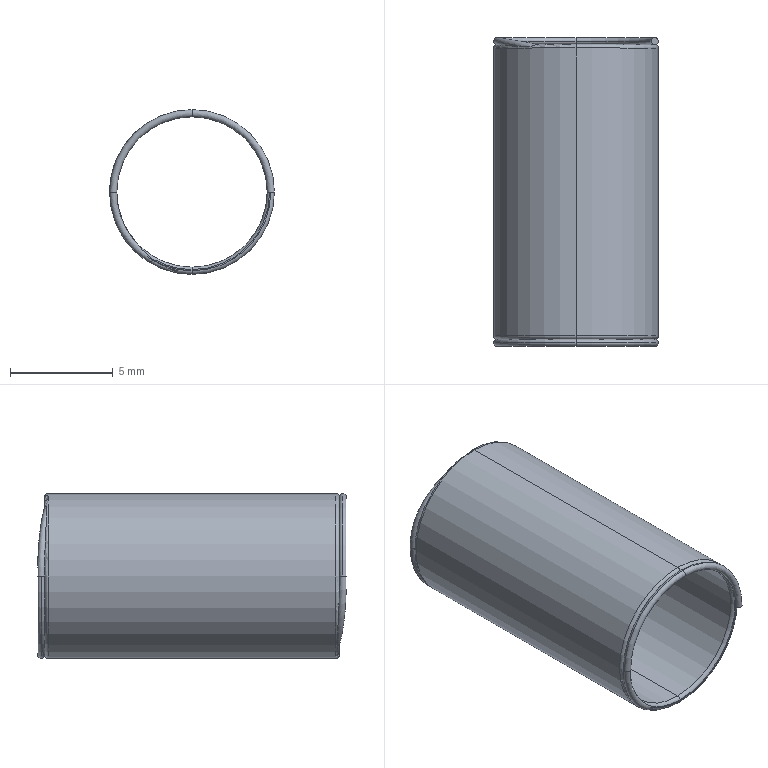Part | STEP file | 11-UF8-15-A11_UV8-15 | 1 solid | 30 faces | box 8 x 15 x 8 mm | volume 122.558 mm3 | torus 22 | cylinder 4 | plane 4 | commonest cylinder face diameters 7.3 x2 8 x2
STEP:
#1=CARTESIAN_POINT('',(0.,-7.325,4.));
#2=VERTEX_POINT('',#1);
#3=CARTESIAN_POINT('',(0.,-7.325,3.65));
#4=VERTEX_POINT('',#3);
#5=CARTESIAN_POINT('',(0.,-7.325,3.825));
#6=DIRECTION('',(1.,0.,0.));
#7=DIRECTION('',(0.,0.,-1.));
#8=AXIS2_PLACEMENT_3D('',#5,#6,#7);
#9=CIRCLE('',#8,0.175);
#10=EDGE_CURVE('',#2,#4,#9,.T.);
#11=ORIENTED_EDGE('',*,*,#10,.F.);
#12=CARTESIAN_POINT('',(-4.,-7.325,0.));
#13=VERTEX_POINT('',#12);
#14=CARTESIAN_POINT('',(0.,-7.325,0.));
#15=DIRECTION('',(0.,-1.,0.));
#16=DIRECTION('',(0.,0.,-1.));
#17=AXIS2_PLACEMENT_3D('',#14,#15,#16);
#18=CIRCLE('',#17,4.);
#19=EDGE_CURVE('',#2,#13,#18,.T.);
#20=ORIENTED_EDGE('',*,*,#19,.T.);
#21=CARTESIAN_POINT('',(-3.65,-7.325,0.));
#22=VERTEX_POINT('',#21);
#23=CARTESIAN_POINT('',(-3.825,-7.325,0.));
#24=DIRECTION('',(0.,0.,1.));
#25=DIRECTION('',(1.,0.,0.));
#26=AXIS2_PLACEMENT_3D('',#23,#24,#25);
#27=CIRCLE('',#26,0.175);
#28=EDGE_CURVE('',#13,#22,#27,.T.);
#29=ORIENTED_EDGE('',*,*,#28,.T.);
#30=CARTESIAN_POINT('',(0.,-7.325,0.));
#31=DIRECTION('',(0.,-1.,0.));
#32=DIRECTION('',(0.,0.,-1.));
#33=AXIS2_PLACEMENT_3D('',#30,#31,#32);
#34=CIRCLE('',#33,3.65);
#35=EDGE_CURVE('',#4,#22,#34,.T.);
#36=ORIENTED_EDGE('',*,*,#35,.F.);
#37=EDGE_LOOP('',(#11,#20,#29,#36));
#38=FACE_OUTER_BOUND('',#37,.T.);
#39=CARTESIAN_POINT('',(0.,-7.325,0.));
#40=DIRECTION('',(0.,-1.,0.));
#41=DIRECTION('',(0.,0.,-1.));
#42=AXIS2_PLACEMENT_3D('',#39,#40,#41);
#43=TOROIDAL_SURFACE('',#42,3.825,0.175);
#44=ADVANCED_FACE('',(#38),#43,.T.);
#45=CARTESIAN_POINT('',(0.,-7.15,3.825));
#46=VERTEX_POINT('',#45);
#47=CARTESIAN_POINT('',(0.,-7.325,3.825));
#48=DIRECTION('',(1.,0.,0.));
#49=DIRECTION('',(0.,0.,-1.));
#50=AXIS2_PLACEMENT_3D('',#47,#48,#49);
#51=CIRCLE('',#50,0.175);
#52=EDGE_CURVE('',#4,#46,#51,.T.);
#53=ORIENTED_EDGE('',*,*,#52,.F.);
#54=ORIENTED_EDGE('',*,*,#35,.T.);
#55=CARTESIAN_POINT('',(-1.895,-7.16,-3.255));
#56=VERTEX_POINT('',#55);
#57=CARTESIAN_POINT('',(-1.895,-7.16,-3.255));
#58=CARTESIAN_POINT('',(-1.953,-7.167,-3.2));
#59=CARTESIAN_POINT('',(-2.014,-7.173,-3.149));
#60=CARTESIAN_POINT('',(-2.136,-7.185,-3.045));
#61=CARTESIAN_POINT('',(-2.196,-7.191,-2.993));
#62=CARTESIAN_POINT('',(-2.374,-7.209,-2.833));
#63=CARTESIAN_POINT('',(-2.489,-7.22,-2.722));
#64=CARTESIAN_POINT('',(-2.814,-7.25,-2.37));
#65=CARTESIAN_POINT('',(-3.006,-7.267,-2.111));
#66=CARTESIAN_POINT('',(-3.319,-7.296,-1.555));
#67=CARTESIAN_POINT('',(-3.442,-7.307,-1.257));
#68=CARTESIAN_POINT('',(-3.566,-7.318,-0.7933));
#69=CARTESIAN_POINT('',(-3.598,-7.32,-0.6364));
#70=CARTESIAN_POINT('',(-3.64,-7.324,-0.3186));
#71=CARTESIAN_POINT('',(-3.65,-7.325,-0.1566));
#72=CARTESIAN_POINT('',(-3.65,-7.325,0.));
#73=B_SPLINE_CURVE_WITH_KNOTS('',3,(#57,#58,#59,#60,#61,#62,#63,#64,#65,#66,#67,#68,#69,#70,#71,#72),.UNSPECIFIED.,.F.,.F.,(4,2,2,2,2,2,2,4),(0.003435,0.00367,0.003905,0.004375,0.005314,0.006254,0.006724,0.007194),.UNSPECIFIED.);
#74=EDGE_CURVE('',#56,#22,#73,.T.);
#75=ORIENTED_EDGE('',*,*,#74,.F.);
#76=CARTESIAN_POINT('',(0.,-7.16,-3.767));
#77=VERTEX_POINT('',#76);
#78=CARTESIAN_POINT('',(0.,-7.16,0.));
#79=DIRECTION('',(0.,-1.,0.));
#80=DIRECTION('',(0.,0.,-1.));
#81=AXIS2_PLACEMENT_3D('',#78,#79,#80);
#82=CIRCLE('',#81,3.767);
#83=EDGE_CURVE('',#56,#77,#82,.T.);
#84=ORIENTED_EDGE('',*,*,#83,.T.);
#85=CARTESIAN_POINT('',(0.,-7.15,-3.825));
#86=VERTEX_POINT('',#85);
#87=CARTESIAN_POINT('',(0.,-7.325,-3.825));
#88=DIRECTION('',(-1.,0.,0.));
#89=DIRECTION('',(0.,0.,1.));
#90=AXIS2_PLACEMENT_3D('',#87,#88,#89);
#91=CIRCLE('',#90,0.175);
#92=EDGE_CURVE('',#77,#86,#91,.T.);
#93=ORIENTED_EDGE('',*,*,#92,.T.);
#94=CARTESIAN_POINT('',(0.,-7.15,0.));
#95=DIRECTION('',(0.,1.,0.));
#96=DIRECTION('',(0.,0.,1.));
#97=AXIS2_PLACEMENT_3D('',#94,#95,#96);
#98=CIRCLE('',#97,3.825);
#99=EDGE_CURVE('',#86,#46,#98,.T.);
#100=ORIENTED_EDGE('',*,*,#99,.T.);
#101=EDGE_LOOP('',(#53,#54,#75,#84,#93,#100));
#102=FACE_OUTER_BOUND('',#101,.T.);
#103=CARTESIAN_POINT('',(0.,-7.325,0.));
#104=DIRECTION('',(0.,-1.,0.));
#105=DIRECTION('',(0.,0.,-1.));
#106=AXIS2_PLACEMENT_3D('',#103,#104,#105);
#107=TOROIDAL_SURFACE('',#106,3.825,0.175);
#108=ADVANCED_FACE('',(#102),#107,.T.);
#109=CARTESIAN_POINT('',(0.,7.325,-4.));
#110=VERTEX_POINT('',#109);
#111=CARTESIAN_POINT('',(0.,7.325,-3.65));
#112=VERTEX_POINT('',#111);
#113=CARTESIAN_POINT('',(0.,7.325,-3.825));
#114=DIRECTION('',(1.,0.,0.));
#115=DIRECTION('',(0.,0.,-1.));
#116=AXIS2_PLACEMENT_3D('',#113,#114,#115);
#117=CIRCLE('',#116,0.175);
#118=EDGE_CURVE('',#110,#112,#117,.T.);
#119=ORIENTED_EDGE('',*,*,#118,.F.);
#120=CARTESIAN_POINT('',(-4.,7.325,0.));
#121=VERTEX_POINT('',#120);
#122=CARTESIAN_POINT('',(0.,7.325,0.));
#123=DIRECTION('',(0.,1.,0.));
#124=DIRECTION('',(0.,0.,1.));
#125=AXIS2_PLACEMENT_3D('',#122,#123,#124);
#126=CIRCLE('',#125,4.);
#127=EDGE_CURVE('',#110,#121,#126,.T.);
#128=ORIENTED_EDGE('',*,*,#127,.T.);
#129=CARTESIAN_POINT('',(-3.65,7.325,0.));
#130=VERTEX_POINT('',#129);
#131=CARTESIAN_POINT('',(-3.825,7.325,0.));
#132=DIRECTION('',(0.,0.,1.));
#133=DIRECTION('',(1.,0.,0.));
#134=AXIS2_PLACEMENT_3D('',#131,#132,#133);
#135=CIRCLE('',#134,0.175);
#136=EDGE_CURVE('',#130,#121,#135,.T.);
#137=ORIENTED_EDGE('',*,*,#136,.F.);
#138=CARTESIAN_POINT('',(0.,7.325,0.));
#139=DIRECTION('',(0.,1.,0.));
#140=DIRECTION('',(0.,0.,1.));
#141=AXIS2_PLACEMENT_3D('',#138,#139,#140);
#142=CIRCLE('',#141,3.65);
#143=EDGE_CURVE('',#112,#130,#142,.T.);
#144=ORIENTED_EDGE('',*,*,#143,.F.);
#145=EDGE_LOOP('',(#119,#128,#137,#144));
#146=FACE_OUTER_BOUND('',#145,.T.);
#147=CARTESIAN_POINT('',(0.,7.325,0.));
#148=DIRECTION('',(0.,1.,0.));
#149=DIRECTION('',(0.,0.,1.));
#150=AXIS2_PLACEMENT_3D('',#147,#148,#149);
#151=TOROIDAL_SURFACE('',#150,3.825,0.175);
#152=ADVANCED_FACE('',(#146),#151,.T.);
#153=CARTESIAN_POINT('',(0.,7.15,-3.825));
#154=VERTEX_POINT('',#153);
#155=CARTESIAN_POINT('',(0.,7.325,-3.825));
#156=DIRECTION('',(1.,0.,0.));
#157=DIRECTION('',(0.,0.,-1.));
#158=AXIS2_PLACEMENT_3D('',#155,#156,#157);
#159=CIRCLE('',#158,0.175);
#160=EDGE_CURVE('',#112,#154,#159,.T.);
#161=ORIENTED_EDGE('',*,*,#160,.F.);
#162=ORIENTED_EDGE('',*,*,#143,.T.);
#163=CARTESIAN_POINT('',(-1.895,7.16,3.255));
#164=VERTEX_POINT('',#163);
#165=CARTESIAN_POINT('',(-3.65,7.325,0.));
#166=CARTESIAN_POINT('',(-3.65,7.325,0.3204));
#167=CARTESIAN_POINT('',(-3.608,7.321,0.6403));
#168=CARTESIAN_POINT('',(-3.442,7.307,1.259));
#169=CARTESIAN_POINT('',(-3.319,7.296,1.556));
#170=CARTESIAN_POINT('',(-3.005,7.267,2.112));
#171=CARTESIAN_POINT('',(-2.814,7.25,2.37));
#172=CARTESIAN_POINT('',(-2.489,7.22,2.722));
#173=CARTESIAN_POINT('',(-2.374,7.209,2.833));
#174=CARTESIAN_POINT('',(-2.196,7.191,2.993));
#175=CARTESIAN_POINT('',(-2.136,7.185,3.046));
#176=CARTESIAN_POINT('',(-2.014,7.173,3.149));
#177=CARTESIAN_POINT('',(-1.953,7.167,3.2));
#178=CARTESIAN_POINT('',(-1.895,7.16,3.255));
#179=B_SPLINE_CURVE_WITH_KNOTS('',3,(#165,#166,#167,#168,#169,#170,#171,#172,#173,#174,#175,#176,#177,#178),.UNSPECIFIED.,.F.,.F.,(4,2,2,2,2,2,4),(-0.0000868,0.0008745,0.001836,0.002797,0.003278,0.003518,0.003758),.UNSPECIFIED.);
#180=EDGE_CURVE('',#130,#164,#179,.T.);
#181=ORIENTED_EDGE('',*,*,#180,.T.);
#182=CARTESIAN_POINT('',(0.,7.16,3.767));
#183=VERTEX_POINT('',#182);
#184=CARTESIAN_POINT('',(0.,7.16,0.));
#185=DIRECTION('',(0.,1.,0.));
#186=DIRECTION('',(0.,0.,1.));
#187=AXIS2_PLACEMENT_3D('',#184,#185,#186);
#188=CIRCLE('',#187,3.767);
#189=EDGE_CURVE('',#164,#183,#188,.T.);
#190=ORIENTED_EDGE('',*,*,#189,.T.);
#191=CARTESIAN_POINT('',(0.,7.15,3.825));
#192=VERTEX_POINT('',#191);
#193=CARTESIAN_POINT('',(0.,7.325,3.825));
#194=DIRECTION('',(-1.,0.,0.));
#195=DIRECTION('',(0.,0.,1.));
#196=AXIS2_PLACEMENT_3D('',#193,#194,#195);
#197=CIRCLE('',#196,0.175);
#198=EDGE_CURVE('',#183,#192,#197,.T.);
#199=ORIENTED_EDGE('',*,*,#198,.T.);
#200=CARTESIAN_POINT('',(0.,7.15,0.));
#201=DIRECTION('',(0.,1.,0.));
#202=DIRECTION('',(0.,0.,1.));
#203=AXIS2_PLACEMENT_3D('',#200,#201,#202);
#204=CIRCLE('',#203,3.825);
#205=EDGE_CURVE('',#154,#192,#204,.T.);
#206=ORIENTED_EDGE('',*,*,#205,.F.);
#207=EDGE_LOOP('',(#161,#162,#181,#190,#199,#206));
#208=FACE_OUTER_BOUND('',#207,.T.);
#209=CARTESIAN_POINT('',(0.,7.325,0.));
#210=DIRECTION('',(0.,1.,0.));
#211=DIRECTION('',(0.,0.,1.));
#212=AXIS2_PLACEMENT_3D('',#209,#210,#211);
#213=TOROIDAL_SURFACE('',#212,3.825,0.175);
#214=ADVANCED_FACE('',(#208),#213,.T.);
#215=CARTESIAN_POINT('',(3.65,7.325,0.));
#216=VERTEX_POINT('',#215);
#217=CARTESIAN_POINT('',(4.,7.325,0.));
#218=VERTEX_POINT('',#217);
#219=CARTESIAN_POINT('',(3.825,7.325,0.));
#220=DIRECTION('',(0.,0.,-1.));
#221=DIRECTION('',(-1.,0.,0.));
#222=AXIS2_PLACEMENT_3D('',#219,#220,#221);
#223=CIRCLE('',#222,0.175);
#224=EDGE_CURVE('',#216,#218,#223,.T.);
#225=ORIENTED_EDGE('',*,*,#224,.T.);
#226=CARTESIAN_POINT('',(0.,7.325,0.));
#227=DIRECTION('',(0.,1.,0.));
#228=DIRECTION('',(0.,0.,1.));
#229=AXIS2_PLACEMENT_3D('',#226,#227,#228);
#230=CIRCLE('',#229,4.);
#231=EDGE_CURVE('',#218,#110,#230,.T.);
#232=ORIENTED_EDGE('',*,*,#231,.T.);
#233=ORIENTED_EDGE('',*,*,#118,.T.);
#234=CARTESIAN_POINT('',(0.,7.325,0.));
#235=DIRECTION('',(0.,1.,0.));
#236=DIRECTION('',(0.,0.,1.));
#237=AXIS2_PLACEMENT_3D('',#234,#235,#236);
#238=CIRCLE('',#237,3.65);
#239=EDGE_CURVE('',#216,#112,#238,.T.);
#240=ORIENTED_EDGE('',*,*,#239,.F.);
#241=EDGE_LOOP('',(#225,#232,#233,#240));
#242=FACE_OUTER_BOUND('',#241,.T.);
#243=CARTESIAN_POINT('',(0.,7.325,0.));
#244=DIRECTION('',(0.,1.,0.));
#245=DIRECTION('',(0.,0.,1.));
#246=AXIS2_PLACEMENT_3D('',#243,#244,#245);
#247=TOROIDAL_SURFACE('',#246,3.825,0.175);
#248=ADVANCED_FACE('',(#242),#247,.T.);
#249=CARTESIAN_POINT('',(3.767,7.16,0.));
#250=VERTEX_POINT('',#249);
#251=CARTESIAN_POINT('',(3.825,7.325,0.));
#252=DIRECTION('',(0.,0.,-1.));
#253=DIRECTION('',(-1.,0.,0.));
#254=AXIS2_PLACEMENT_3D('',#251,#252,#253);
#255=CIRCLE('',#254,0.175);
#256=EDGE_CURVE('',#250,#216,#255,.T.);
#257=ORIENTED_EDGE('',*,*,#256,.T.);
#258=ORIENTED_EDGE('',*,*,#239,.T.);
#259=ORIENTED_EDGE('',*,*,#160,.T.);
#260=CARTESIAN_POINT('',(0.,7.15,0.));
#261=DIRECTION('',(0.,1.,0.));
#262=DIRECTION('',(0.,0.,1.));
#263=AXIS2_PLACEMENT_3D('',#260,#261,#262);
#264=CIRCLE('',#263,3.825);
#265=EDGE_CURVE('',#192,#154,#264,.T.);
#266=ORIENTED_EDGE('',*,*,#265,.F.);
#267=ORIENTED_EDGE('',*,*,#198,.F.);
#268=CARTESIAN_POINT('',(0.,7.16,0.));
#269=DIRECTION('',(0.,1.,0.));
#270=DIRECTION('',(0.,0.,1.));
#271=AXIS2_PLACEMENT_3D('',#268,#269,#270);
#272=CIRCLE('',#271,3.767);
#273=EDGE_CURVE('',#183,#250,#272,.T.);
#274=ORIENTED_EDGE('',*,*,#273,.T.);
#275=EDGE_LOOP('',(#257,#258,#259,#266,#267,#274));
#276=FACE_OUTER_BOUND('',#275,.T.);
#277=CARTESIAN_POINT('',(0.,7.325,0.));
#278=DIRECTION('',(0.,1.,0.));
#279=DIRECTION('',(0.,0.,1.));
#280=AXIS2_PLACEMENT_3D('',#277,#278,#279);
#281=TOROIDAL_SURFACE('',#280,3.825,0.175);
#282=ADVANCED_FACE('',(#276),#281,.T.);
#283=CARTESIAN_POINT('',(4.,-7.325,0.));
#284=VERTEX_POINT('',#283);
#285=CARTESIAN_POINT('',(3.65,-7.325,0.));
#286=VERTEX_POINT('',#285);
#287=CARTESIAN_POINT('',(3.825,-7.325,0.));
#288=DIRECTION('',(0.,0.,-1.));
#289=DIRECTION('',(-1.,0.,0.));
#290=AXIS2_PLACEMENT_3D('',#287,#288,#289);
#291=CIRCLE('',#290,0.175);
#292=EDGE_CURVE('',#284,#286,#291,.T.);
#293=ORIENTED_EDGE('',*,*,#292,.F.);
#294=CARTESIAN_POINT('',(0.,-7.325,0.));
#295=DIRECTION('',(0.,-1.,0.));
#296=DIRECTION('',(0.,0.,-1.));
#297=AXIS2_PLACEMENT_3D('',#294,#295,#296);
#298=CIRCLE('',#297,4.);
#299=EDGE_CURVE('',#284,#2,#298,.T.);
#300=ORIENTED_EDGE('',*,*,#299,.T.);
#301=ORIENTED_EDGE('',*,*,#10,.T.);
#302=CARTESIAN_POINT('',(0.,-7.325,0.));
#303=DIRECTION('',(0.,-1.,0.));
#304=DIRECTION('',(0.,0.,-1.));
#305=AXIS2_PLACEMENT_3D('',#302,#303,#304);
#306=CIRCLE('',#305,3.65);
#307=EDGE_CURVE('',#286,#4,#306,.T.);
#308=ORIENTED_EDGE('',*,*,#307,.F.);
#309=EDGE_LOOP('',(#293,#300,#301,#308));
#310=FACE_OUTER_BOUND('',#309,.T.);
#311=CARTESIAN_POINT('',(0.,-7.325,0.));
#312=DIRECTION('',(0.,-1.,0.));
#313=DIRECTION('',(0.,0.,-1.));
#314=AXIS2_PLACEMENT_3D('',#311,#312,#313);
#315=TOROIDAL_SURFACE('',#314,3.825,0.175);
#316=ADVANCED_FACE('',(#310),#315,.T.);
#317=CARTESIAN_POINT('',(3.767,-7.16,0.));
#318=VERTEX_POINT('',#317);
#319=CARTESIAN_POINT('',(3.825,-7.325,0.));
#320=DIRECTION('',(0.,0.,-1.));
#321=DIRECTION('',(-1.,0.,0.));
#322=AXIS2_PLACEMENT_3D('',#319,#320,#321);
#323=CIRCLE('',#322,0.175);
#324=EDGE_CURVE('',#286,#318,#323,.T.);
#325=ORIENTED_EDGE('',*,*,#324,.F.);
#326=ORIENTED_EDGE('',*,*,#307,.T.);
#327=ORIENTED_EDGE('',*,*,#52,.T.);
#328=CARTESIAN_POINT('',(0.,-7.15,0.));
#329=DIRECTION('',(0.,1.,0.));
#330=DIRECTION('',(0.,0.,1.));
#331=AXIS2_PLACEMENT_3D('',#328,#329,#330);
#332=CIRCLE('',#331,3.825);
#333=EDGE_CURVE('',#46,#86,#332,.T.);
#334=ORIENTED_EDGE('',*,*,#333,.T.);
#335=ORIENTED_EDGE('',*,*,#92,.F.);
#336=CARTESIAN_POINT('',(0.,-7.16,0.));
#337=DIRECTION('',(0.,-1.,0.));
#338=DIRECTION('',(0.,0.,-1.));
#339=AXIS2_PLACEMENT_3D('',#336,#337,#338);
#340=CIRCLE('',#339,3.767);
#341=EDGE_CURVE('',#77,#318,#340,.T.);
#342=ORIENTED_EDGE('',*,*,#341,.T.);
#343=EDGE_LOOP('',(#325,#326,#327,#334,#335,#342));
#344=FACE_OUTER_BOUND('',#343,.T.);
#345=CARTESIAN_POINT('',(0.,-7.325,0.));
#346=DIRECTION('',(0.,-1.,0.));
#347=DIRECTION('',(0.,0.,-1.));
#348=AXIS2_PLACEMENT_3D('',#345,#346,#347);
#349=TOROIDAL_SURFACE('',#348,3.825,0.175);
#350=ADVANCED_FACE('',(#344),#349,.T.);
#351=ORIENTED_EDGE('',*,*,#265,.T.);
#352=CARTESIAN_POINT('',(0.,6.975,-3.65));
#353=VERTEX_POINT('',#352);
#354=CARTESIAN_POINT('',(0.,6.975,-3.825));
#355=DIRECTION('',(1.,0.,0.));
#356=DIRECTION('',(0.,0.,-1.));
#357=AXIS2_PLACEMENT_3D('',#354,#355,#356);
#358=CIRCLE('',#357,0.175);
#359=EDGE_CURVE('',#154,#353,#358,.T.);
#360=ORIENTED_EDGE('',*,*,#359,.T.);
#361=CARTESIAN_POINT('',(0.,6.975,3.65));
#362=VERTEX_POINT('',#361);
#363=CARTESIAN_POINT('',(0.,6.975,0.));
#364=DIRECTION('',(0.,1.,0.));
#365=DIRECTION('',(0.,0.,1.));
#366=AXIS2_PLACEMENT_3D('',#363,#364,#365);
#367=CIRCLE('',#366,3.65);
#368=EDGE_CURVE('',#362,#353,#367,.T.);
#369=ORIENTED_EDGE('',*,*,#368,.F.);
#370=CARTESIAN_POINT('',(0.,6.975,3.825));
#371=DIRECTION('',(-1.,0.,0.));
#372=DIRECTION('',(0.,0.,1.));
#373=AXIS2_PLACEMENT_3D('',#370,#371,#372);
#374=CIRCLE('',#373,0.175);
#375=EDGE_CURVE('',#192,#362,#374,.T.);
#376=ORIENTED_EDGE('',*,*,#375,.F.);
#377=EDGE_LOOP('',(#351,#360,#369,#376));
#378=FACE_OUTER_BOUND('',#377,.T.);
#379=CARTESIAN_POINT('',(0.,6.975,0.));
#380=DIRECTION('',(0.,1.,0.));
#381=DIRECTION('',(0.,0.,1.));
#382=AXIS2_PLACEMENT_3D('',#379,#380,#381);
#383=TOROIDAL_SURFACE('',#382,3.825,0.175);
#384=ADVANCED_FACE('',(#378),#383,.T.);
#385=CARTESIAN_POINT('',(0.,-6.975,-3.65));
#386=VERTEX_POINT('',#385);
#387=CARTESIAN_POINT('',(0.,-6.975,3.65));
#388=VERTEX_POINT('',#387);
#389=CARTESIAN_POINT('',(0.,-6.975,0.));
#390=DIRECTION('',(0.,1.,0.));
#391=DIRECTION('',(0.,0.,1.));
#392=AXIS2_PLACEMENT_3D('',#389,#390,#391);
#393=CIRCLE('',#392,3.65);
#394=EDGE_CURVE('',#386,#388,#393,.T.);
#395=ORIENTED_EDGE('',*,*,#394,.F.);
#396=CARTESIAN_POINT('',(0.,-7.5,-3.65));
#397=DIRECTION('',(0.,1.,0.));
#398=VECTOR('',#397,1000.);
#399=LINE('',#396,#398);
#400=EDGE_CURVE('',#386,#353,#399,.T.);
#401=ORIENTED_EDGE('',*,*,#400,.T.);
#402=CARTESIAN_POINT('',(0.,6.975,0.));
#403=DIRECTION('',(0.,1.,0.));
#404=DIRECTION('',(0.,0.,1.));
#405=AXIS2_PLACEMENT_3D('',#402,#403,#404);
#406=CIRCLE('',#405,3.65);
#407=EDGE_CURVE('',#353,#362,#406,.T.);
#408=ORIENTED_EDGE('',*,*,#407,.T.);
#409=CARTESIAN_POINT('',(0.,-7.5,3.65));
#410=DIRECTION('',(0.,1.,0.));
#411=VECTOR('',#410,1000.);
#412=LINE('',#409,#411);
#413=EDGE_CURVE('',#388,#362,#412,.T.);
#414=ORIENTED_EDGE('',*,*,#413,.F.);
#415=EDGE_LOOP('',(#395,#401,#408,#414));
#416=FACE_OUTER_BOUND('',#415,.T.);
#417=CARTESIAN_POINT('',(0.,-7.5,0.));
#418=DIRECTION('',(0.,1.,0.));
#419=DIRECTION('',(0.,0.,1.));
#420=AXIS2_PLACEMENT_3D('',#417,#418,#419);
#421=CYLINDRICAL_SURFACE('',#420,3.65);
#422=ADVANCED_FACE('',(#416),#421,.F.);
#423=CARTESIAN_POINT('',(0.,-6.975,0.));
#424=DIRECTION('',(0.,1.,0.));
#425=DIRECTION('',(0.,0.,1.));
#426=AXIS2_PLACEMENT_3D('',#423,#424,#425);
#427=CIRCLE('',#426,3.65);
#428=EDGE_CURVE('',#388,#386,#427,.T.);
#429=ORIENTED_EDGE('',*,*,#428,.T.);
#430=CARTESIAN_POINT('',(0.,-6.975,-3.825));
#431=DIRECTION('',(1.,0.,0.));
#432=DIRECTION('',(0.,0.,-1.));
#433=AXIS2_PLACEMENT_3D('',#430,#431,#432);
#434=CIRCLE('',#433,0.175);
#435=EDGE_CURVE('',#386,#86,#434,.T.);
#436=ORIENTED_EDGE('',*,*,#435,.T.);
#437=ORIENTED_EDGE('',*,*,#333,.F.);
#438=CARTESIAN_POINT('',(0.,-6.975,3.825));
#439=DIRECTION('',(-1.,0.,0.));
#440=DIRECTION('',(0.,0.,1.));
#441=AXIS2_PLACEMENT_3D('',#438,#439,#440);
#442=CIRCLE('',#441,0.175);
#443=EDGE_CURVE('',#388,#46,#442,.T.);
#444=ORIENTED_EDGE('',*,*,#443,.F.);
#445=EDGE_LOOP('',(#429,#436,#437,#444));
#446=FACE_OUTER_BOUND('',#445,.T.);
#447=CARTESIAN_POINT('',(0.,-6.975,0.));
#448=DIRECTION('',(0.,1.,0.));
#449=DIRECTION('',(0.,0.,1.));
#450=AXIS2_PLACEMENT_3D('',#447,#448,#449);
#451=TOROIDAL_SURFACE('',#450,3.825,0.175);
#452=ADVANCED_FACE('',(#446),#451,.T.);
#453=ORIENTED_EDGE('',*,*,#299,.F.);
#454=CARTESIAN_POINT('',(3.867,-7.155,0.));
#455=VERTEX_POINT('',#454);
#456=CARTESIAN_POINT('',(3.825,-7.325,0.));
#457=DIRECTION('',(0.,0.,-1.));
#458=DIRECTION('',(-1.,0.,0.));
#459=AXIS2_PLACEMENT_3D('',#456,#457,#458);
#460=CIRCLE('',#459,0.175);
#461=EDGE_CURVE('',#455,#284,#460,.T.);
#462=ORIENTED_EDGE('',*,*,#461,.F.);
#463=CARTESIAN_POINT('',(0.,-7.155,3.867));
#464=VERTEX_POINT('',#463);
#465=CARTESIAN_POINT('',(0.,-7.155,0.));
#466=DIRECTION('',(0.,-1.,0.));
#467=DIRECTION('',(0.,0.,-1.));
#468=AXIS2_PLACEMENT_3D('',#465,#466,#467);
#469=CIRCLE('',#468,3.867);
#470=EDGE_CURVE('',#455,#464,#469,.T.);
#471=ORIENTED_EDGE('',*,*,#470,.T.);
#472=CARTESIAN_POINT('',(0.,-7.325,3.825));
#473=DIRECTION('',(1.,0.,0.));
#474=DIRECTION('',(0.,0.,-1.));
#475=AXIS2_PLACEMENT_3D('',#472,#473,#474);
#476=CIRCLE('',#475,0.175);
#477=EDGE_CURVE('',#464,#2,#476,.T.);
#478=ORIENTED_EDGE('',*,*,#477,.T.);
#479=EDGE_LOOP('',(#453,#462,#471,#478));
#480=FACE_OUTER_BOUND('',#479,.T.);
#481=CARTESIAN_POINT('',(0.,-7.325,0.));
#482=DIRECTION('',(0.,-1.,0.));
#483=DIRECTION('',(0.,0.,-1.));
#484=AXIS2_PLACEMENT_3D('',#481,#482,#483);
#485=TOROIDAL_SURFACE('',#484,3.825,0.175);
#486=ADVANCED_FACE('',(#480),#485,.T.);
#487=ORIENTED_EDGE('',*,*,#231,.F.);
#488=CARTESIAN_POINT('',(3.867,7.155,0.));
#489=VERTEX_POINT('',#488);
#490=CARTESIAN_POINT('',(3.825,7.325,0.));
#491=DIRECTION('',(0.,0.,-1.));
#492=DIRECTION('',(-1.,0.,0.));
#493=AXIS2_PLACEMENT_3D('',#490,#491,#492);
#494=CIRCLE('',#493,0.175);
#495=EDGE_CURVE('',#218,#489,#494,.T.);
#496=ORIENTED_EDGE('',*,*,#495,.T.);
#497=CARTESIAN_POINT('',(0.,7.155,-3.867));
#498=VERTEX_POINT('',#497);
#499=CARTESIAN_POINT('',(0.,7.155,0.));
#500=DIRECTION('',(0.,-1.,0.));
#501=DIRECTION('',(0.,0.,1.));
#502=AXIS2_PLACEMENT_3D('',#499,#500,#501);
#503=CIRCLE('',#502,3.867);
#504=EDGE_CURVE('',#498,#489,#503,.T.);
#505=ORIENTED_EDGE('',*,*,#504,.F.);
#506=CARTESIAN_POINT('',(0.,7.325,-3.825));
#507=DIRECTION('',(1.,0.,0.));
#508=DIRECTION('',(0.,0.,-1.));
#509=AXIS2_PLACEMENT_3D('',#506,#507,#508);
#510=CIRCLE('',#509,0.175);
#511=EDGE_CURVE('',#498,#110,#510,.T.);
#512=ORIENTED_EDGE('',*,*,#511,.T.);
#513=EDGE_LOOP('',(#487,#496,#505,#512));
#514=FACE_OUTER_BOUND('',#513,.T.);
#515=CARTESIAN_POINT('',(0.,7.325,0.));
#516=DIRECTION('',(0.,1.,0.));
#517=DIRECTION('',(0.,0.,1.));
#518=AXIS2_PLACEMENT_3D('',#515,#516,#517);
#519=TOROIDAL_SURFACE('',#518,3.825,0.175);
#520=ADVANCED_FACE('',(#514),#519,.T.);
#521=CARTESIAN_POINT('',(3.825,-7.16,0.));
#522=VERTEX_POINT('',#521);
#523=CARTESIAN_POINT('',(0.,-7.16,-3.825));
#524=VERTEX_POINT('',#523);
#525=CARTESIAN_POINT('',(0.,-7.16,0.));
#526=DIRECTION('',(0.,1.,0.));
#527=DIRECTION('',(0.,0.,1.));
#528=AXIS2_PLACEMENT_3D('',#525,#526,#527);
#529=CIRCLE('',#528,3.825);
#530=EDGE_CURVE('',#522,#524,#529,.T.);
#531=ORIENTED_EDGE('',*,*,#530,.T.);
#532=CARTESIAN_POINT('',(0.,-6.985,-4.));
#533=VERTEX_POINT('',#532);
#534=CARTESIAN_POINT('',(0.,-6.985,-3.825));
#535=DIRECTION('',(1.,0.,0.));
#536=DIRECTION('',(0.,0.,-1.));
#537=AXIS2_PLACEMENT_3D('',#534,#535,#536);
#538=CIRCLE('',#537,0.175);
#539=EDGE_CURVE('',#524,#533,#538,.T.);
#540=ORIENTED_EDGE('',*,*,#539,.T.);
#541=CARTESIAN_POINT('',(0.,-6.985,4.));
#542=VERTEX_POINT('',#541);
#543=CARTESIAN_POINT('',(0.,-6.985,0.));
#544=DIRECTION('',(0.,1.,0.));
#545=DIRECTION('',(0.,0.,1.));
#546=AXIS2_PLACEMENT_3D('',#543,#544,#545);
#547=CIRCLE('',#546,4.);
#548=EDGE_CURVE('',#542,#533,#547,.T.);
#549=ORIENTED_EDGE('',*,*,#548,.F.);
#550=CARTESIAN_POINT('',(0.,-6.985,3.825));
#551=DIRECTION('',(-1.,0.,0.));
#552=DIRECTION('',(0.,0.,1.));
#553=AXIS2_PLACEMENT_3D('',#550,#551,#552);
#554=CIRCLE('',#553,0.175);
#555=EDGE_CURVE('',#464,#542,#554,.T.);
#556=ORIENTED_EDGE('',*,*,#555,.F.);
#557=ORIENTED_EDGE('',*,*,#470,.F.);
#558=CARTESIAN_POINT('',(3.825,-6.985,0.));
#559=DIRECTION('',(0.,0.,-1.));
#560=DIRECTION('',(-1.,0.,0.));
#561=AXIS2_PLACEMENT_3D('',#558,#559,#560);
#562=CIRCLE('',#561,0.175);
#563=EDGE_CURVE('',#455,#522,#562,.T.);
#564=ORIENTED_EDGE('',*,*,#563,.T.);
#565=EDGE_LOOP('',(#531,#540,#549,#556,#557,#564));
#566=FACE_OUTER_BOUND('',#565,.T.);
#567=CARTESIAN_POINT('',(0.,-6.985,0.));
#568=DIRECTION('',(0.,1.,0.));
#569=DIRECTION('',(0.,0.,1.));
#570=AXIS2_PLACEMENT_3D('',#567,#568,#569);
#571=TOROIDAL_SURFACE('',#570,3.825,0.175);
#572=ADVANCED_FACE('',(#566),#571,.T.);
#573=ORIENTED_EDGE('',*,*,#548,.T.);
#574=CARTESIAN_POINT('',(0.,6.985,-4.));
#575=VERTEX_POINT('',#574);
#576=CARTESIAN_POINT('',(0.,-7.16,-4.));
#577=DIRECTION('',(0.,1.,0.));
#578=VECTOR('',#577,1000.);
#579=LINE('',#576,#578);
#580=EDGE_CURVE('',#533,#575,#579,.T.);
#581=ORIENTED_EDGE('',*,*,#580,.T.);
#582=CARTESIAN_POINT('',(0.,6.985,4.));
#583=VERTEX_POINT('',#582);
#584=CARTESIAN_POINT('',(0.,6.985,0.));
#585=DIRECTION('',(0.,1.,0.));
#586=DIRECTION('',(0.,0.,1.));
#587=AXIS2_PLACEMENT_3D('',#584,#585,#586);
#588=CIRCLE('',#587,4.);
#589=EDGE_CURVE('',#583,#575,#588,.T.);
#590=ORIENTED_EDGE('',*,*,#589,.F.);
#591=CARTESIAN_POINT('',(0.,-7.16,4.));
#592=DIRECTION('',(0.,1.,0.));
#593=VECTOR('',#592,1000.);
#594=LINE('',#591,#593);
#595=EDGE_CURVE('',#542,#583,#594,.T.);
#596=ORIENTED_EDGE('',*,*,#595,.F.);
#597=EDGE_LOOP('',(#573,#581,#590,#596));
#598=FACE_OUTER_BOUND('',#597,.T.);
#599=CARTESIAN_POINT('',(0.,-7.16,0.));
#600=DIRECTION('',(0.,1.,0.));
#601=DIRECTION('',(0.,0.,1.));
#602=AXIS2_PLACEMENT_3D('',#599,#600,#601);
#603=CYLINDRICAL_SURFACE('',#602,4.);
#604=ADVANCED_FACE('',(#598),#603,.T.);
#605=ORIENTED_EDGE('',*,*,#589,.T.);
#606=CARTESIAN_POINT('',(0.,6.985,-3.825));
#607=DIRECTION('',(1.,0.,0.));
#608=DIRECTION('',(0.,0.,-1.));
#609=AXIS2_PLACEMENT_3D('',#606,#607,#608);
#610=CIRCLE('',#609,0.175);
#611=EDGE_CURVE('',#575,#498,#610,.T.);
#612=ORIENTED_EDGE('',*,*,#611,.T.);
#613=ORIENTED_EDGE('',*,*,#504,.T.);
#614=CARTESIAN_POINT('',(3.825,7.16,0.));
#615=VERTEX_POINT('',#614);
#616=CARTESIAN_POINT('',(3.825,6.985,0.));
#617=DIRECTION('',(0.,0.,-1.));
#618=DIRECTION('',(-1.,0.,0.));
#619=AXIS2_PLACEMENT_3D('',#616,#617,#618);
#620=CIRCLE('',#619,0.175);
#621=EDGE_CURVE('',#615,#489,#620,.T.);
#622=ORIENTED_EDGE('',*,*,#621,.F.);
#623=CARTESIAN_POINT('',(0.,7.16,3.825));
#624=VERTEX_POINT('',#623);
#625=CARTESIAN_POINT('',(0.,7.16,0.));
#626=DIRECTION('',(0.,1.,0.));
#627=DIRECTION('',(0.,0.,1.));
#628=AXIS2_PLACEMENT_3D('',#625,#626,#627);
#629=CIRCLE('',#628,3.825);
#630=EDGE_CURVE('',#624,#615,#629,.T.);
#631=ORIENTED_EDGE('',*,*,#630,.F.);
#632=CARTESIAN_POINT('',(0.,6.985,3.825));
#633=DIRECTION('',(-1.,0.,0.));
#634=DIRECTION('',(0.,0.,1.));
#635=AXIS2_PLACEMENT_3D('',#632,#633,#634);
#636=CIRCLE('',#635,0.175);
#637=EDGE_CURVE('',#583,#624,#636,.T.);
#638=ORIENTED_EDGE('',*,*,#637,.F.);
#639=EDGE_LOOP('',(#605,#612,#613,#622,#631,#638));
#640=FACE_OUTER_BOUND('',#639,.T.);
#641=CARTESIAN_POINT('',(0.,6.985,0.));
#642=DIRECTION('',(0.,1.,0.));
#643=DIRECTION('',(0.,0.,1.));
#644=AXIS2_PLACEMENT_3D('',#641,#642,#643);
#645=TOROIDAL_SURFACE('',#644,3.825,0.175);
#646=ADVANCED_FACE('',(#640),#645,.T.);
#647=ORIENTED_EDGE('',*,*,#180,.F.);
#648=ORIENTED_EDGE('',*,*,#136,.T.);
#649=CARTESIAN_POINT('',(-3.867,7.155,0.));
#650=VERTEX_POINT('',#649);
#651=CARTESIAN_POINT('',(-3.825,7.325,0.));
#652=DIRECTION('',(0.,0.,1.));
#653=DIRECTION('',(1.,0.,0.));
#654=AXIS2_PLACEMENT_3D('',#651,#652,#653);
#655=CIRCLE('',#654,0.175);
#656=EDGE_CURVE('',#121,#650,#655,.T.);
#657=ORIENTED_EDGE('',*,*,#656,.T.);
#658=CARTESIAN_POINT('',(-1.896,7.16,3.322));
#659=VERTEX_POINT('',#658);
#660=CARTESIAN_POINT('',(-3.867,7.155,0.));
#661=CARTESIAN_POINT('',(-3.867,7.155,0.3545));
#662=CARTESIAN_POINT('',(-3.835,7.151,0.7083));
#663=CARTESIAN_POINT('',(-3.719,7.138,1.219));
#664=CARTESIAN_POINT('',(-3.669,7.133,1.387));
#665=CARTESIAN_POINT('',(-3.545,7.122,1.717));
#666=CARTESIAN_POINT('',(-3.471,7.115,1.879));
#667=CARTESIAN_POINT('',(-3.219,7.092,2.341));
#668=CARTESIAN_POINT('',(-3.012,7.074,2.621));
#669=CARTESIAN_POINT('',(-2.636,7.05,2.997));
#670=CARTESIAN_POINT('',(-2.502,7.041,3.115));
#671=CARTESIAN_POINT('',(-2.322,7.044,3.245));
#672=CARTESIAN_POINT('',(-2.285,7.046,3.27));
#673=CARTESIAN_POINT('',(-2.21,7.054,3.317));
#674=CARTESIAN_POINT('',(-2.172,7.061,3.339));
#675=CARTESIAN_POINT('',(-2.093,7.086,3.372));
#676=CARTESIAN_POINT('',(-2.053,7.107,3.38));
#677=CARTESIAN_POINT('',(-1.974,7.145,3.366));
#678=CARTESIAN_POINT('',(-1.934,7.16,3.345));
#679=CARTESIAN_POINT('',(-1.896,7.16,3.322));
#680=B_SPLINE_CURVE_WITH_KNOTS('',3,(#660,#661,#662,#663,#664,#665,#666,#667,#668,#669,#670,#671,#672,#673,#674,#675,#676,#677,#678,#679),.UNSPECIFIED.,.F.,.F.,(4,2,2,2,2,2,2,2,2,4),(0.0000002,0.001063,0.001595,0.002126,0.003189,0.003721,0.003854,0.003987,0.004119,0.004252),.UNSPECIFIED.);
#681=EDGE_CURVE('',#650,#659,#680,.T.);
#682=ORIENTED_EDGE('',*,*,#681,.T.);
#683=CARTESIAN_POINT('',(-1.896,7.16,3.322));
#684=CARTESIAN_POINT('',(-1.886,7.16,3.315));
#685=CARTESIAN_POINT('',(-1.88,7.16,3.302));
#686=CARTESIAN_POINT('',(-1.883,7.16,3.278));
#687=CARTESIAN_POINT('',(-1.889,7.16,3.266));
#688=CARTESIAN_POINT('',(-1.895,7.16,3.255));
#689=B_SPLINE_CURVE_WITH_KNOTS('',3,(#683,#684,#685,#686,#687,#688),.UNSPECIFIED.,.F.,.F.,(4,2,4),(0.01652,0.01656,0.0166),.UNSPECIFIED.);
#690=EDGE_CURVE('',#659,#164,#689,.T.);
#691=ORIENTED_EDGE('',*,*,#690,.T.);
#692=EDGE_LOOP('',(#647,#648,#657,#682,#691));
#693=FACE_OUTER_BOUND('',#692,.T.);
#694=CARTESIAN_POINT('',(-0.1153,6.671,0.));
#695=DIRECTION('',(-0.1736,-0.9848,0.));
#696=DIRECTION('',(0.9848,-0.1736,0.));
#697=AXIS2_PLACEMENT_3D('',#694,#695,#696);
#698=TOROIDAL_SURFACE('',#697,3.767,0.175);
#699=ADVANCED_FACE('',(#693),#698,.T.);
#700=CARTESIAN_POINT('',(-1.896,-7.16,-3.322));
#701=VERTEX_POINT('',#700);
#702=CARTESIAN_POINT('',(-1.895,-7.16,-3.255));
#703=CARTESIAN_POINT('',(-1.889,-7.16,-3.266));
#704=CARTESIAN_POINT('',(-1.883,-7.16,-3.277));
#705=CARTESIAN_POINT('',(-1.88,-7.16,-3.302));
#706=CARTESIAN_POINT('',(-1.886,-7.16,-3.315));
#707=CARTESIAN_POINT('',(-1.896,-7.16,-3.322));
#708=B_SPLINE_CURVE_WITH_KNOTS('',3,(#702,#703,#704,#705,#706,#707),.UNSPECIFIED.,.F.,.F.,(4,2,4),(0.01641,0.01645,0.01649),.UNSPECIFIED.);
#709=EDGE_CURVE('',#56,#701,#708,.T.);
#710=ORIENTED_EDGE('',*,*,#709,.F.);
#711=ORIENTED_EDGE('',*,*,#74,.T.);
#712=ORIENTED_EDGE('',*,*,#28,.F.);
#713=CARTESIAN_POINT('',(-3.867,-7.155,0.));
#714=VERTEX_POINT('',#713);
#715=CARTESIAN_POINT('',(-3.825,-7.325,0.));
#716=DIRECTION('',(0.,0.,1.));
#717=DIRECTION('',(1.,0.,0.));
#718=AXIS2_PLACEMENT_3D('',#715,#716,#717);
#719=CIRCLE('',#718,0.175);
#720=EDGE_CURVE('',#714,#13,#719,.T.);
#721=ORIENTED_EDGE('',*,*,#720,.F.);
#722=CARTESIAN_POINT('',(-1.896,-7.16,-3.322));
#723=CARTESIAN_POINT('',(-1.935,-7.16,-3.345));
#724=CARTESIAN_POINT('',(-1.974,-7.146,-3.366));
#725=CARTESIAN_POINT('',(-2.053,-7.107,-3.38));
#726=CARTESIAN_POINT('',(-2.094,-7.086,-3.372));
#727=CARTESIAN_POINT('',(-2.173,-7.061,-3.339));
#728=CARTESIAN_POINT('',(-2.211,-7.054,-3.316));
#729=CARTESIAN_POINT('',(-2.286,-7.046,-3.27));
#730=CARTESIAN_POINT('',(-2.322,-7.044,-3.244));
#731=CARTESIAN_POINT('',(-2.502,-7.041,-3.114));
#732=CARTESIAN_POINT('',(-2.635,-7.05,-2.999));
#733=CARTESIAN_POINT('',(-3.006,-7.074,-2.627));
#734=CARTESIAN_POINT('',(-3.22,-7.092,-2.34));
#735=CARTESIAN_POINT('',(-3.555,-7.122,-1.724));
#736=CARTESIAN_POINT('',(-3.68,-7.134,-1.389));
#737=CARTESIAN_POINT('',(-3.836,-7.151,-0.7062));
#738=CARTESIAN_POINT('',(-3.867,-7.155,-0.3537));
#739=CARTESIAN_POINT('',(-3.867,-7.155,0.));
#740=B_SPLINE_CURVE_WITH_KNOTS('',3,(#722,#723,#724,#725,#726,#727,#728,#729,#730,#731,#732,#733,#734,#735,#736,#737,#738,#739),.UNSPECIFIED.,.F.,.F.,(4,2,2,2,2,2,2,2,4),(0.0006315,0.0007642,0.000897,0.00103,0.001163,0.001694,0.002756,0.003818,0.00488),.UNSPECIFIED.);
#741=EDGE_CURVE('',#701,#714,#740,.T.);
#742=ORIENTED_EDGE('',*,*,#741,.F.);
#743=EDGE_LOOP('',(#710,#711,#712,#721,#742));
#744=FACE_OUTER_BOUND('',#743,.T.);
#745=CARTESIAN_POINT('',(-0.1153,-6.671,0.));
#746=DIRECTION('',(-0.1736,0.9848,0.));
#747=DIRECTION('',(-0.9848,-0.1736,0.));
#748=AXIS2_PLACEMENT_3D('',#745,#746,#747);
#749=TOROIDAL_SURFACE('',#748,3.767,0.175);
#750=ADVANCED_FACE('',(#744),#749,.T.);
#751=ORIENTED_EDGE('',*,*,#189,.F.);
#752=ORIENTED_EDGE('',*,*,#690,.F.);
#753=CARTESIAN_POINT('',(0.,7.16,0.));
#754=DIRECTION('',(0.,1.,0.));
#755=DIRECTION('',(0.,0.,1.));
#756=AXIS2_PLACEMENT_3D('',#753,#754,#755);
#757=CIRCLE('',#756,3.825);
#758=EDGE_CURVE('',#659,#624,#757,.T.);
#759=ORIENTED_EDGE('',*,*,#758,.T.);
#760=ORIENTED_EDGE('',*,*,#630,.T.);
#761=CARTESIAN_POINT('',(0.,7.16,0.));
#762=DIRECTION('',(1.,0.,0.));
#763=VECTOR('',#762,1000.);
#764=LINE('',#761,#763);
#765=EDGE_CURVE('',#250,#615,#764,.T.);
#766=ORIENTED_EDGE('',*,*,#765,.F.);
#767=ORIENTED_EDGE('',*,*,#273,.F.);
#768=EDGE_LOOP('',(#751,#752,#759,#760,#766,#767));
#769=FACE_OUTER_BOUND('',#768,.T.);
#770=CARTESIAN_POINT('',(0.,7.16,0.));
#771=DIRECTION('',(0.,-1.,0.));
#772=DIRECTION('',(0.,0.,-1.));
#773=AXIS2_PLACEMENT_3D('',#770,#771,#772);
#774=PLANE('',#773);
#775=ADVANCED_FACE('',(#769),#774,.F.);
#776=ORIENTED_EDGE('',*,*,#611,.F.);
#777=CARTESIAN_POINT('',(0.,6.985,0.));
#778=DIRECTION('',(0.,1.,0.));
#779=DIRECTION('',(0.,0.,1.));
#780=AXIS2_PLACEMENT_3D('',#777,#778,#779);
#781=CIRCLE('',#780,4.);
#782=EDGE_CURVE('',#575,#583,#781,.T.);
#783=ORIENTED_EDGE('',*,*,#782,.T.);
#784=ORIENTED_EDGE('',*,*,#637,.T.);
#785=ORIENTED_EDGE('',*,*,#758,.F.);
#786=ORIENTED_EDGE('',*,*,#681,.F.);
#787=CARTESIAN_POINT('',(0.,7.155,0.));
#788=DIRECTION('',(0.,-1.,0.));
#789=DIRECTION('',(0.,0.,1.));
#790=AXIS2_PLACEMENT_3D('',#787,#788,#789);
#791=CIRCLE('',#790,3.867);
#792=EDGE_CURVE('',#650,#498,#791,.T.);
#793=ORIENTED_EDGE('',*,*,#792,.T.);
#794=EDGE_LOOP('',(#776,#783,#784,#785,#786,#793));
#795=FACE_OUTER_BOUND('',#794,.T.);
#796=CARTESIAN_POINT('',(0.,6.985,0.));
#797=DIRECTION('',(0.,1.,0.));
#798=DIRECTION('',(0.,0.,1.));
#799=AXIS2_PLACEMENT_3D('',#796,#797,#798);
#800=TOROIDAL_SURFACE('',#799,3.825,0.175);
#801=ADVANCED_FACE('',(#795),#800,.T.);
#802=ORIENTED_EDGE('',*,*,#580,.F.);
#803=CARTESIAN_POINT('',(0.,-6.985,0.));
#804=DIRECTION('',(0.,1.,0.));
#805=DIRECTION('',(0.,0.,1.));
#806=AXIS2_PLACEMENT_3D('',#803,#804,#805);
#807=CIRCLE('',#806,4.);
#808=EDGE_CURVE('',#533,#542,#807,.T.);
#809=ORIENTED_EDGE('',*,*,#808,.T.);
#810=ORIENTED_EDGE('',*,*,#595,.T.);
#811=ORIENTED_EDGE('',*,*,#782,.F.);
#812=EDGE_LOOP('',(#802,#809,#810,#811));
#813=FACE_OUTER_BOUND('',#812,.T.);
#814=CARTESIAN_POINT('',(0.,-7.16,0.));
#815=DIRECTION('',(0.,1.,0.));
#816=DIRECTION('',(0.,0.,1.));
#817=AXIS2_PLACEMENT_3D('',#814,#815,#816);
#818=CYLINDRICAL_SURFACE('',#817,4.);
#819=ADVANCED_FACE('',(#813),#818,.T.);
#820=ORIENTED_EDGE('',*,*,#539,.F.);
#821=CARTESIAN_POINT('',(0.,-7.16,0.));
#822=DIRECTION('',(0.,1.,0.));
#823=DIRECTION('',(0.,0.,1.));
#824=AXIS2_PLACEMENT_3D('',#821,#822,#823);
#825=CIRCLE('',#824,3.825);
#826=EDGE_CURVE('',#524,#701,#825,.T.);
#827=ORIENTED_EDGE('',*,*,#826,.T.);
#828=ORIENTED_EDGE('',*,*,#741,.T.);
#829=CARTESIAN_POINT('',(0.,-7.155,0.));
#830=DIRECTION('',(0.,-1.,0.));
#831=DIRECTION('',(0.,0.,-1.));
#832=AXIS2_PLACEMENT_3D('',#829,#830,#831);
#833=CIRCLE('',#832,3.867);
#834=EDGE_CURVE('',#464,#714,#833,.T.);
#835=ORIENTED_EDGE('',*,*,#834,.F.);
#836=ORIENTED_EDGE('',*,*,#555,.T.);
#837=ORIENTED_EDGE('',*,*,#808,.F.);
#838=EDGE_LOOP('',(#820,#827,#828,#835,#836,#837));
#839=FACE_OUTER_BOUND('',#838,.T.);
#840=CARTESIAN_POINT('',(0.,-6.985,0.));
#841=DIRECTION('',(0.,1.,0.));
#842=DIRECTION('',(0.,0.,1.));
#843=AXIS2_PLACEMENT_3D('',#840,#841,#842);
#844=TOROIDAL_SURFACE('',#843,3.825,0.175);
#845=ADVANCED_FACE('',(#839),#844,.T.);
#846=ORIENTED_EDGE('',*,*,#83,.F.);
#847=ORIENTED_EDGE('',*,*,#709,.T.);
#848=ORIENTED_EDGE('',*,*,#826,.F.);
#849=ORIENTED_EDGE('',*,*,#530,.F.);
#850=CARTESIAN_POINT('',(3.825,-7.16,0.));
#851=DIRECTION('',(-1.,0.,0.));
#852=VECTOR('',#851,1000.);
#853=LINE('',#850,#852);
#854=EDGE_CURVE('',#522,#318,#853,.T.);
#855=ORIENTED_EDGE('',*,*,#854,.T.);
#856=ORIENTED_EDGE('',*,*,#341,.F.);
#857=EDGE_LOOP('',(#846,#847,#848,#849,#855,#856));
#858=FACE_OUTER_BOUND('',#857,.T.);
#859=CARTESIAN_POINT('',(3.825,-7.16,0.));
#860=DIRECTION('',(0.,1.,0.));
#861=DIRECTION('',(0.,0.,1.));
#862=AXIS2_PLACEMENT_3D('',#859,#860,#861);
#863=PLANE('',#862);
#864=ADVANCED_FACE('',(#858),#863,.F.);
#865=ORIENTED_EDGE('',*,*,#127,.F.);
#866=ORIENTED_EDGE('',*,*,#511,.F.);
#867=ORIENTED_EDGE('',*,*,#792,.F.);
#868=ORIENTED_EDGE('',*,*,#656,.F.);
#869=EDGE_LOOP('',(#865,#866,#867,#868));
#870=FACE_OUTER_BOUND('',#869,.T.);
#871=CARTESIAN_POINT('',(0.,7.325,0.));
#872=DIRECTION('',(0.,1.,0.));
#873=DIRECTION('',(0.,0.,1.));
#874=AXIS2_PLACEMENT_3D('',#871,#872,#873);
#875=TOROIDAL_SURFACE('',#874,3.825,0.175);
#876=ADVANCED_FACE('',(#870),#875,.T.);
#877=ORIENTED_EDGE('',*,*,#256,.F.);
#878=ORIENTED_EDGE('',*,*,#765,.T.);
#879=ORIENTED_EDGE('',*,*,#621,.T.);
#880=ORIENTED_EDGE('',*,*,#495,.F.);
#881=ORIENTED_EDGE('',*,*,#224,.F.);
#882=EDGE_LOOP('',(#877,#878,#879,#880,#881));
#883=FACE_OUTER_BOUND('',#882,.T.);
#884=CARTESIAN_POINT('',(3.825,7.325,0.));
#885=DIRECTION('',(0.,0.,-1.));
#886=DIRECTION('',(-1.,0.,0.));
#887=AXIS2_PLACEMENT_3D('',#884,#885,#886);
#888=PLANE('',#887);
#889=ADVANCED_FACE('',(#883),#888,.F.);
#890=ORIENTED_EDGE('',*,*,#19,.F.);
#891=ORIENTED_EDGE('',*,*,#477,.F.);
#892=ORIENTED_EDGE('',*,*,#834,.T.);
#893=ORIENTED_EDGE('',*,*,#720,.T.);
#894=EDGE_LOOP('',(#890,#891,#892,#893));
#895=FACE_OUTER_BOUND('',#894,.T.);
#896=CARTESIAN_POINT('',(0.,-7.325,0.));
#897=DIRECTION('',(0.,-1.,0.));
#898=DIRECTION('',(0.,0.,-1.));
#899=AXIS2_PLACEMENT_3D('',#896,#897,#898);
#900=TOROIDAL_SURFACE('',#899,3.825,0.175);
#901=ADVANCED_FACE('',(#895),#900,.T.);
#902=ORIENTED_EDGE('',*,*,#563,.F.);
#903=ORIENTED_EDGE('',*,*,#461,.T.);
#904=ORIENTED_EDGE('',*,*,#292,.T.);
#905=ORIENTED_EDGE('',*,*,#324,.T.);
#906=ORIENTED_EDGE('',*,*,#854,.F.);
#907=EDGE_LOOP('',(#902,#903,#904,#905,#906));
#908=FACE_OUTER_BOUND('',#907,.T.);
#909=CARTESIAN_POINT('',(3.825,-7.325,0.));
#910=DIRECTION('',(0.,0.,-1.));
#911=DIRECTION('',(-1.,0.,0.));
#912=AXIS2_PLACEMENT_3D('',#909,#910,#911);
#913=PLANE('',#912);
#914=ADVANCED_FACE('',(#908),#913,.T.);
#915=ORIENTED_EDGE('',*,*,#435,.F.);
#916=ORIENTED_EDGE('',*,*,#394,.T.);
#917=ORIENTED_EDGE('',*,*,#443,.T.);
#918=ORIENTED_EDGE('',*,*,#99,.F.);
#919=EDGE_LOOP('',(#915,#916,#917,#918));
#920=FACE_OUTER_BOUND('',#919,.T.);
#921=CARTESIAN_POINT('',(0.,-6.975,0.));
#922=DIRECTION('',(0.,1.,0.));
#923=DIRECTION('',(0.,0.,1.));
#924=AXIS2_PLACEMENT_3D('',#921,#922,#923);
#925=TOROIDAL_SURFACE('',#924,3.825,0.175);
#926=ADVANCED_FACE('',(#920),#925,.T.);
#927=ORIENTED_EDGE('',*,*,#400,.F.);
#928=ORIENTED_EDGE('',*,*,#428,.F.);
#929=ORIENTED_EDGE('',*,*,#413,.T.);
#930=ORIENTED_EDGE('',*,*,#368,.T.);
#931=EDGE_LOOP('',(#927,#928,#929,#930));
#932=FACE_OUTER_BOUND('',#931,.T.);
#933=CARTESIAN_POINT('',(0.,-7.5,0.));
#934=DIRECTION('',(0.,1.,0.));
#935=DIRECTION('',(0.,0.,1.));
#936=AXIS2_PLACEMENT_3D('',#933,#934,#935);
#937=CYLINDRICAL_SURFACE('',#936,3.65);
#938=ADVANCED_FACE('',(#932),#937,.F.);
#939=ORIENTED_EDGE('',*,*,#359,.F.);
#940=ORIENTED_EDGE('',*,*,#205,.T.);
#941=ORIENTED_EDGE('',*,*,#375,.T.);
#942=ORIENTED_EDGE('',*,*,#407,.F.);
#943=EDGE_LOOP('',(#939,#940,#941,#942));
#944=FACE_OUTER_BOUND('',#943,.T.);
#945=CARTESIAN_POINT('',(0.,6.975,0.));
#946=DIRECTION('',(0.,1.,0.));
#947=DIRECTION('',(0.,0.,1.));
#948=AXIS2_PLACEMENT_3D('',#945,#946,#947);
#949=TOROIDAL_SURFACE('',#948,3.825,0.175);
#950=ADVANCED_FACE('',(#944),#949,.T.);
#951=CLOSED_SHELL('',(#44,#108,#152,#214,#248,#282,#316,#350,#384,#422,#452,#486,#520,#572,#604,#646,#699,#750,#775,#801,#819,#845,#864,#876,#889,#901,#914,#926,#938,#950));
#952=MANIFOLD_SOLID_BREP('',#951);
#953=CARTESIAN_POINT('',(0.,0.,0.));
#954=DIRECTION('',(0.,0.,1.));
#955=DIRECTION('',(1.,0.,0.));
#956=AXIS2_PLACEMENT_3D('',#953,#954,#955);
#957=(LENGTH_UNIT()NAMED_UNIT(*)SI_UNIT(.MILLI.,.METRE.));
#958=UNCERTAINTY_MEASURE_WITH_UNIT(LENGTH_MEASURE(0.00001),#957,'','');
#959=(NAMED_UNIT(*)PLANE_ANGLE_UNIT()SI_UNIT($,.RADIAN.));
#960=(NAMED_UNIT(*)SI_UNIT($,.STERADIAN.)SOLID_ANGLE_UNIT());
#961=(GEOMETRIC_REPRESENTATION_CONTEXT(3)GLOBAL_UNCERTAINTY_ASSIGNED_CONTEXT((#958))GLOBAL_UNIT_ASSIGNED_CONTEXT((#957,#959,#960))REPRESENTATION_CONTEXT('',''));
#962=ADVANCED_BREP_SHAPE_REPRESENTATION('',(#952,#956),#961);